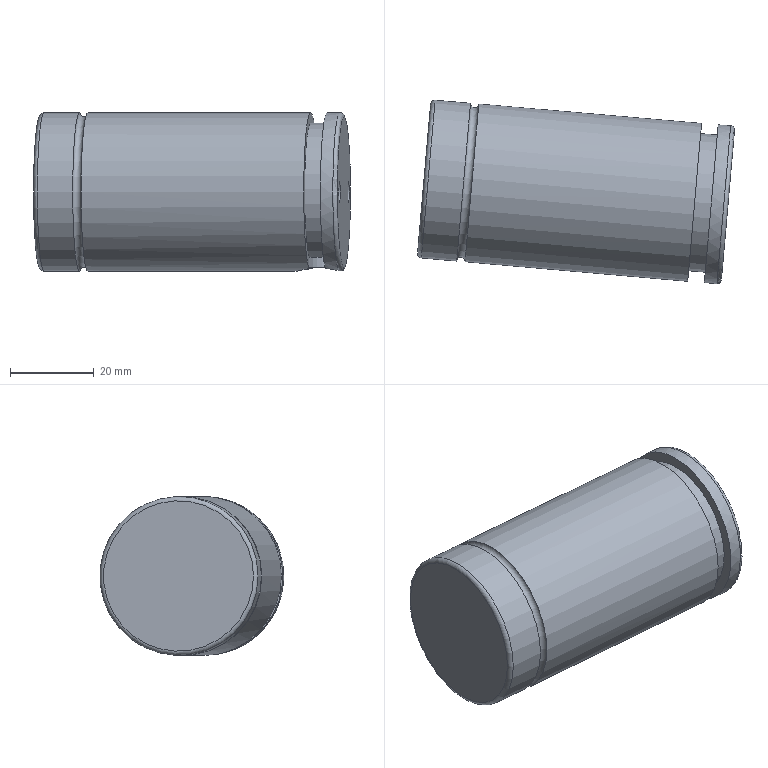Part | NX | features solid 2 | 1 solid | 26 faces | box 75.867 x 44.051 x 38 mm | volume 81103 mm3 | plane 13 | cylinder 8 | torus 3 | cone 2 | commonest cylinder face diameters 38 x3 4.9 x2 9.5 x1 11 x1 33 x1
STEP:
#1=CARTESIAN_POINT('',(-732.743,476.677,-245.));
#2=VERTEX_POINT('',#1);
#3=CARTESIAN_POINT('',(-731.087,495.604,-245.));
#4=DIRECTION('',(-0.9962,0.08716,0.));
#5=DIRECTION('',(-0.08716,-0.9962,0.));
#6=AXIS2_PLACEMENT_3D('',#3,#4,#5);
#7=CIRCLE('',#6,19.);
#8=EDGE_CURVE('',#2,#2,#7,.T.);
#9=ORIENTED_EDGE('',*,*,#8,.T.);
#10=EDGE_LOOP('',(#9));
#11=FACE_BOUND('',#10,.T.);
#12=CARTESIAN_POINT('',(-734.736,476.851,-245.));
#13=VERTEX_POINT('',#12);
#14=CARTESIAN_POINT('',(-733.08,495.779,-245.));
#15=DIRECTION('',(-0.9962,0.08716,0.));
#16=DIRECTION('',(-0.08716,-0.9962,0.));
#17=AXIS2_PLACEMENT_3D('',#14,#15,#16);
#18=CIRCLE('',#17,19.);
#19=EDGE_CURVE('',#13,#13,#18,.T.);
#20=ORIENTED_EDGE('',*,*,#19,.F.);
#21=EDGE_LOOP('',(#20));
#22=FACE_BOUND('',#21,.T.);
#23=CARTESIAN_POINT('',(-732.083,495.692,-245.));
#24=DIRECTION('',(-0.9962,0.08716,0.));
#25=DIRECTION('',(0.,0.,-1.));
#26=AXIS2_PLACEMENT_3D('',#23,#24,#25);
#27=TOROIDAL_SURFACE('',#26,19.,1.);
#28=ADVANCED_FACE('',(#11,#22),#27,.F.);
#29=CARTESIAN_POINT('',(-743.203,477.592,-245.));
#30=VERTEX_POINT('',#29);
#31=CARTESIAN_POINT('',(-741.547,496.52,-245.));
#32=DIRECTION('',(-0.9962,0.08716,0.));
#33=DIRECTION('',(-0.08716,-0.9962,0.));
#34=AXIS2_PLACEMENT_3D('',#31,#32,#33);
#35=CIRCLE('',#34,19.);
#36=EDGE_CURVE('',#30,#30,#35,.T.);
#37=ORIENTED_EDGE('',*,*,#36,.T.);
#38=EDGE_LOOP('',(#37));
#39=FACE_BOUND('',#38,.T.);
#40=CARTESIAN_POINT('',(-744.112,478.675,-245.));
#41=VERTEX_POINT('',#40);
#42=CARTESIAN_POINT('',(-742.543,496.607,-245.));
#43=DIRECTION('',(-0.9962,0.08716,0.));
#44=DIRECTION('',(-0.08716,-0.9962,0.));
#45=AXIS2_PLACEMENT_3D('',#42,#43,#44);
#46=CIRCLE('',#45,18.);
#47=EDGE_CURVE('',#41,#41,#46,.T.);
#48=ORIENTED_EDGE('',*,*,#47,.F.);
#49=EDGE_LOOP('',(#48));
#50=FACE_BOUND('',#49,.T.);
#51=CARTESIAN_POINT('',(-741.547,496.52,-245.));
#52=DIRECTION('',(-0.9962,0.08716,0.));
#53=DIRECTION('',(0.,0.,-1.));
#54=AXIS2_PLACEMENT_3D('',#51,#52,#53);
#55=TOROIDAL_SURFACE('',#54,18.,1.);
#56=ADVANCED_FACE('',(#39,#50),#55,.T.);
#57=ORIENTED_EDGE('',*,*,#19,.T.);
#58=EDGE_LOOP('',(#57));
#59=FACE_BOUND('',#58,.T.);
#60=ORIENTED_EDGE('',*,*,#36,.F.);
#61=EDGE_LOOP('',(#60));
#62=FACE_BOUND('',#61,.T.);
#63=CARTESIAN_POINT('',(-737.313,496.149,-245.));
#64=DIRECTION('',(0.9962,-0.08716,0.));
#65=DIRECTION('',(0.,0.,1.));
#66=AXIS2_PLACEMENT_3D('',#63,#64,#65);
#67=CYLINDRICAL_SURFACE('',#66,19.);
#68=ADVANCED_FACE('',(#59,#62),#67,.T.);
#69=CARTESIAN_POINT('',(-678.237,485.838,-260.684));
#70=VERTEX_POINT('',#69);
#71=CARTESIAN_POINT('',(-677.344,496.046,-260.684));
#72=VERTEX_POINT('',#71);
#73=CARTESIAN_POINT('',(-677.791,490.942,-245.));
#74=DIRECTION('',(-0.9962,0.08716,0.));
#75=DIRECTION('',(-0.08716,-0.9962,0.));
#76=AXIS2_PLACEMENT_3D('',#73,#74,#75);
#77=CIRCLE('',#76,16.5);
#78=EDGE_CURVE('',#70,#72,#77,.T.);
#79=ORIENTED_EDGE('',*,*,#78,.F.);
#80=CARTESIAN_POINT('',(-674.253,485.489,-260.684));
#81=VERTEX_POINT('',#80);
#82=CARTESIAN_POINT('',(-678.237,485.838,-260.684));
#83=CARTESIAN_POINT('',(-677.01,485.23,-260.522));
#84=CARTESIAN_POINT('',(-675.567,485.104,-260.522));
#85=CARTESIAN_POINT('',(-674.253,485.489,-260.684));
#86=B_SPLINE_CURVE_WITH_KNOTS('',3,(#82,#83,#84,#85),.UNSPECIFIED.,.F.,.F.,(4,4),(0.,0.004081),.UNSPECIFIED.);
#87=EDGE_CURVE('',#70,#81,#86,.T.);
#88=ORIENTED_EDGE('',*,*,#87,.T.);
#89=CARTESIAN_POINT('',(-673.36,495.697,-260.684));
#90=VERTEX_POINT('',#89);
#91=CARTESIAN_POINT('',(-673.806,490.593,-245.));
#92=DIRECTION('',(-0.9962,0.08716,0.));
#93=DIRECTION('',(-0.08716,-0.9962,0.));
#94=AXIS2_PLACEMENT_3D('',#91,#92,#93);
#95=CIRCLE('',#94,16.5);
#96=EDGE_CURVE('',#81,#90,#95,.T.);
#97=ORIENTED_EDGE('',*,*,#96,.T.);
#98=CARTESIAN_POINT('',(-673.36,495.697,-260.684));
#99=CARTESIAN_POINT('',(-674.587,496.304,-260.522));
#100=CARTESIAN_POINT('',(-676.03,496.431,-260.522));
#101=CARTESIAN_POINT('',(-677.344,496.046,-260.684));
#102=B_SPLINE_CURVE_WITH_KNOTS('',3,(#98,#99,#100,#101),.UNSPECIFIED.,.F.,.F.,(4,4),(0.,0.004081),.UNSPECIFIED.);
#103=EDGE_CURVE('',#90,#72,#102,.T.);
#104=ORIENTED_EDGE('',*,*,#103,.T.);
#105=EDGE_LOOP('',(#79,#88,#97,#104));
#106=FACE_BOUND('',#105,.T.);
#107=CARTESIAN_POINT('',(-675.798,490.767,-245.));
#108=DIRECTION('',(0.9962,-0.08716,0.));
#109=DIRECTION('',(0.,0.,1.));
#110=AXIS2_PLACEMENT_3D('',#107,#108,#109);
#111=CYLINDRICAL_SURFACE('',#110,16.5);
#112=ADVANCED_FACE('',(#106),#111,.T.);
#113=CARTESIAN_POINT('',(-674.253,485.489,-263.296));
#114=VERTEX_POINT('',#113);
#115=CARTESIAN_POINT('',(-673.36,495.697,-263.296));
#116=VERTEX_POINT('',#115);
#117=CARTESIAN_POINT('',(-673.806,490.593,-245.));
#118=DIRECTION('',(-0.9962,0.08716,0.));
#119=DIRECTION('',(-0.08716,-0.9962,0.));
#120=AXIS2_PLACEMENT_3D('',#117,#118,#119);
#121=CIRCLE('',#120,19.);
#122=EDGE_CURVE('',#114,#116,#121,.T.);
#123=ORIENTED_EDGE('',*,*,#122,.F.);
#124=CARTESIAN_POINT('',(-671.017,488.049,-263.861));
#125=VERTEX_POINT('',#124);
#126=CARTESIAN_POINT('',(-674.253,485.489,-263.296));
#127=CARTESIAN_POINT('',(-672.883,485.89,-263.442));
#128=CARTESIAN_POINT('',(-671.722,486.809,-263.704));
#129=CARTESIAN_POINT('',(-671.017,488.049,-263.861));
#130=B_SPLINE_CURVE_WITH_KNOTS('',3,(#126,#127,#128,#129),.UNSPECIFIED.,.F.,.F.,(4,4),(0.,0.004242),.UNSPECIFIED.);
#131=EDGE_CURVE('',#114,#125,#130,.T.);
#132=ORIENTED_EDGE('',*,*,#131,.T.);
#133=CARTESIAN_POINT('',(-670.618,492.614,-263.861));
#134=VERTEX_POINT('',#133);
#135=CARTESIAN_POINT('',(-670.817,490.331,-245.));
#136=DIRECTION('',(-0.9962,0.08716,0.));
#137=DIRECTION('',(-0.08716,-0.9962,0.));
#138=AXIS2_PLACEMENT_3D('',#135,#136,#137);
#139=CIRCLE('',#138,19.);
#140=EDGE_CURVE('',#125,#134,#139,.T.);
#141=ORIENTED_EDGE('',*,*,#140,.T.);
#142=CARTESIAN_POINT('',(-670.618,492.614,-263.861));
#143=CARTESIAN_POINT('',(-671.097,493.957,-263.704));
#144=CARTESIAN_POINT('',(-672.08,495.064,-263.442));
#145=CARTESIAN_POINT('',(-673.36,495.697,-263.296));
#146=B_SPLINE_CURVE_WITH_KNOTS('',3,(#142,#143,#144,#145),.UNSPECIFIED.,.F.,.F.,(4,4),(0.,0.004242),.UNSPECIFIED.);
#147=EDGE_CURVE('',#134,#116,#146,.T.);
#148=ORIENTED_EDGE('',*,*,#147,.T.);
#149=EDGE_LOOP('',(#123,#132,#141,#148));
#150=FACE_BOUND('',#149,.T.);
#151=CARTESIAN_POINT('',(-672.312,490.462,-245.));
#152=DIRECTION('',(0.9962,-0.08716,0.));
#153=DIRECTION('',(0.,0.,1.));
#154=AXIS2_PLACEMENT_3D('',#151,#152,#153);
#155=CYLINDRICAL_SURFACE('',#154,19.);
#156=ADVANCED_FACE('',(#150),#155,.T.);
#157=CARTESIAN_POINT('',(-670.697,480.233,-245.));
#158=VERTEX_POINT('',#157);
#159=CARTESIAN_POINT('',(-670.911,477.792,-245.));
#160=DIRECTION('',(-0.9962,0.08716,0.));
#161=DIRECTION('',(0.08716,0.9962,0.));
#162=AXIS2_PLACEMENT_3D('',#159,#160,#161);
#163=CIRCLE('',#162,2.45);
#164=EDGE_CURVE('',#158,#158,#163,.T.);
#165=ORIENTED_EDGE('',*,*,#164,.F.);
#166=EDGE_LOOP('',(#165));
#167=FACE_BOUND('',#166,.T.);
#168=CARTESIAN_POINT('',(-677.87,480.86,-245.));
#169=VERTEX_POINT('',#168);
#170=CARTESIAN_POINT('',(-678.083,478.419,-245.));
#171=DIRECTION('',(0.9962,-0.08716,0.));
#172=DIRECTION('',(0.08716,0.9962,0.));
#173=AXIS2_PLACEMENT_3D('',#170,#171,#172);
#174=CIRCLE('',#173,2.45);
#175=EDGE_CURVE('',#169,#169,#174,.T.);
#176=ORIENTED_EDGE('',*,*,#175,.F.);
#177=EDGE_LOOP('',(#176));
#178=FACE_BOUND('',#177,.T.);
#179=CARTESIAN_POINT('',(-674.497,478.106,-245.));
#180=DIRECTION('',(-0.9962,0.08716,0.));
#181=DIRECTION('',(0.,0.,-1.));
#182=AXIS2_PLACEMENT_3D('',#179,#180,#181);
#183=CYLINDRICAL_SURFACE('',#182,2.45);
#184=ADVANCED_FACE('',(#167,#178),#183,.F.);
#185=CARTESIAN_POINT('',(-679.378,478.533,-245.));
#186=VERTEX_POINT('',#185);
#187=VERTEX_LOOP('',#186);
#188=FACE_BOUND('',#187,.T.);
#189=ORIENTED_EDGE('',*,*,#175,.T.);
#190=EDGE_LOOP('',(#189));
#191=FACE_BOUND('',#190,.T.);
#192=CARTESIAN_POINT('',(-678.731,478.476,-245.));
#193=DIRECTION('',(0.9962,-0.08716,0.));
#194=DIRECTION('',(0.,0.,1.));
#195=AXIS2_PLACEMENT_3D('',#192,#193,#194);
#196=CONICAL_SURFACE('',#195,1.225,1.083);
#197=ADVANCED_FACE('',(#188,#191),#196,.F.);
#198=CARTESIAN_POINT('',(-676.118,500.884,-245.));
#199=VERTEX_POINT('',#198);
#200=CARTESIAN_POINT('',(-675.904,503.324,-245.));
#201=DIRECTION('',(-0.9962,0.08716,0.));
#202=DIRECTION('',(-0.08716,-0.9962,0.));
#203=AXIS2_PLACEMENT_3D('',#200,#201,#202);
#204=CIRCLE('',#203,2.45);
#205=EDGE_CURVE('',#199,#199,#204,.T.);
#206=ORIENTED_EDGE('',*,*,#205,.F.);
#207=EDGE_LOOP('',(#206));
#208=FACE_BOUND('',#207,.T.);
#209=CARTESIAN_POINT('',(-677.199,503.438,-245.));
#210=VERTEX_POINT('',#209);
#211=VERTEX_LOOP('',#210);
#212=FACE_BOUND('',#211,.T.);
#213=CARTESIAN_POINT('',(-676.552,503.381,-245.));
#214=DIRECTION('',(0.9962,-0.08716,0.));
#215=DIRECTION('',(0.,0.,1.));
#216=AXIS2_PLACEMENT_3D('',#213,#214,#215);
#217=CONICAL_SURFACE('',#216,1.225,1.083);
#218=ADVANCED_FACE('',(#208,#212),#217,.F.);
#219=ORIENTED_EDGE('',*,*,#205,.T.);
#220=EDGE_LOOP('',(#219));
#221=FACE_BOUND('',#220,.T.);
#222=CARTESIAN_POINT('',(-668.945,500.256,-245.));
#223=VERTEX_POINT('',#222);
#224=CARTESIAN_POINT('',(-668.732,502.697,-245.));
#225=DIRECTION('',(-0.9962,0.08716,0.));
#226=DIRECTION('',(-0.08716,-0.9962,0.));
#227=AXIS2_PLACEMENT_3D('',#224,#225,#226);
#228=CIRCLE('',#227,2.45);
#229=EDGE_CURVE('',#223,#223,#228,.T.);
#230=ORIENTED_EDGE('',*,*,#229,.F.);
#231=EDGE_LOOP('',(#230));
#232=FACE_BOUND('',#231,.T.);
#233=CARTESIAN_POINT('',(-672.318,503.01,-245.));
#234=DIRECTION('',(0.9962,-0.08716,0.));
#235=DIRECTION('',(0.,0.,1.));
#236=AXIS2_PLACEMENT_3D('',#233,#234,#235);
#237=CYLINDRICAL_SURFACE('',#236,2.45);
#238=ADVANCED_FACE('',(#221,#232),#237,.F.);
#239=CARTESIAN_POINT('',(-671.39,472.313,-245.));
#240=VERTEX_POINT('',#239);
#241=CARTESIAN_POINT('',(-669.821,490.244,-245.));
#242=DIRECTION('',(-0.9962,0.08716,0.));
#243=DIRECTION('',(-0.08716,-0.9962,0.));
#244=AXIS2_PLACEMENT_3D('',#241,#242,#243);
#245=CIRCLE('',#244,18.);
#246=EDGE_CURVE('',#240,#240,#245,.T.);
#247=ORIENTED_EDGE('',*,*,#246,.T.);
#248=EDGE_LOOP('',(#247));
#249=FACE_BOUND('',#248,.T.);
#250=CARTESIAN_POINT('',(-671.017,488.049,-263.861));
#251=CARTESIAN_POINT('',(-670.626,488.737,-263.949));
#252=CARTESIAN_POINT('',(-670.15,490.274,-263.783));
#253=CARTESIAN_POINT('',(-670.352,491.868,-263.949));
#254=CARTESIAN_POINT('',(-670.618,492.614,-263.861));
#255=B_SPLINE_CURVE_WITH_KNOTS('',3,(#250,#251,#252,#253,#254),.UNSPECIFIED.,.F.,.F.,(4,1,4),(0.,0.002357,0.004713),.UNSPECIFIED.);
#256=EDGE_CURVE('',#125,#134,#255,.T.);
#257=ORIENTED_EDGE('',*,*,#256,.T.);
#258=ORIENTED_EDGE('',*,*,#140,.F.);
#259=EDGE_LOOP('',(#257,#258));
#260=FACE_BOUND('',#259,.T.);
#261=CARTESIAN_POINT('',(-670.817,490.331,-245.));
#262=DIRECTION('',(-0.9962,0.08716,0.));
#263=DIRECTION('',(0.,0.,-1.));
#264=AXIS2_PLACEMENT_3D('',#261,#262,#263);
#265=TOROIDAL_SURFACE('',#264,18.,1.);
#266=ADVANCED_FACE('',(#249,#260),#265,.T.);
#267=CARTESIAN_POINT('',(-678.237,485.838,-263.296));
#268=VERTEX_POINT('',#267);
#269=CARTESIAN_POINT('',(-677.344,496.046,-263.296));
#270=VERTEX_POINT('',#269);
#271=CARTESIAN_POINT('',(-677.791,490.942,-245.));
#272=DIRECTION('',(-0.9962,0.08716,0.));
#273=DIRECTION('',(-0.08716,-0.9962,0.));
#274=AXIS2_PLACEMENT_3D('',#271,#272,#273);
#275=CIRCLE('',#274,19.);
#276=EDGE_CURVE('',#268,#270,#275,.T.);
#277=ORIENTED_EDGE('',*,*,#276,.T.);
#278=CARTESIAN_POINT('',(-677.344,496.046,-263.296));
#279=CARTESIAN_POINT('',(-678.409,495.734,-263.409));
#280=CARTESIAN_POINT('',(-680.292,494.49,-263.782));
#281=CARTESIAN_POINT('',(-681.623,491.275,-264.109));
#282=CARTESIAN_POINT('',(-680.879,487.899,-263.784));
#283=CARTESIAN_POINT('',(-679.232,486.33,-263.409));
#284=CARTESIAN_POINT('',(-678.237,485.838,-263.296));
#285=B_SPLINE_CURVE_WITH_KNOTS('',3,(#278,#279,#280,#281,#282,#283,#284),.UNSPECIFIED.,.F.,.F.,(4,1,1,1,4),(-0.006599,-0.0033,-0.000001213,0.003297,0.006596),.UNSPECIFIED.);
#286=EDGE_CURVE('',#270,#268,#285,.T.);
#287=ORIENTED_EDGE('',*,*,#286,.T.);
#288=EDGE_LOOP('',(#277,#287));
#289=FACE_BOUND('',#288,.T.);
#290=ORIENTED_EDGE('',*,*,#8,.F.);
#291=EDGE_LOOP('',(#290));
#292=FACE_BOUND('',#291,.T.);
#293=CARTESIAN_POINT('',(-704.439,493.273,-245.));
#294=DIRECTION('',(0.9962,-0.08716,0.));
#295=DIRECTION('',(0.,0.,1.));
#296=AXIS2_PLACEMENT_3D('',#293,#294,#295);
#297=CYLINDRICAL_SURFACE('',#296,19.);
#298=ADVANCED_FACE('',(#289,#292),#297,.T.);
#299=CARTESIAN_POINT('',(-676.278,485.288,-260.5));
#300=VERTEX_POINT('',#299);
#301=CARTESIAN_POINT('',(-675.798,490.767,-260.5));
#302=DIRECTION('',(0.,0.,-1.));
#303=DIRECTION('',(-0.08716,-0.9962,0.));
#304=AXIS2_PLACEMENT_3D('',#301,#302,#303);
#305=CIRCLE('',#304,5.5);
#306=EDGE_CURVE('',#300,#300,#305,.T.);
#307=ORIENTED_EDGE('',*,*,#306,.F.);
#308=EDGE_LOOP('',(#307));
#309=FACE_BOUND('',#308,.T.);
#310=ORIENTED_EDGE('',*,*,#87,.F.);
#311=CARTESIAN_POINT('',(-678.237,485.838,-262.25));
#312=DIRECTION('',(0.,0.,1.));
#313=VECTOR('',#312,1000.);
#314=LINE('',#311,#313);
#315=EDGE_CURVE('',#268,#70,#314,.T.);
#316=ORIENTED_EDGE('',*,*,#315,.F.);
#317=ORIENTED_EDGE('',*,*,#286,.F.);
#318=CARTESIAN_POINT('',(-677.344,496.046,-262.25));
#319=DIRECTION('',(0.,0.,-1.));
#320=VECTOR('',#319,1000.);
#321=LINE('',#318,#320);
#322=EDGE_CURVE('',#72,#270,#321,.T.);
#323=ORIENTED_EDGE('',*,*,#322,.F.);
#324=ORIENTED_EDGE('',*,*,#103,.F.);
#325=CARTESIAN_POINT('',(-673.36,495.697,-262.25));
#326=DIRECTION('',(0.,0.,1.));
#327=VECTOR('',#326,1000.);
#328=LINE('',#325,#327);
#329=EDGE_CURVE('',#116,#90,#328,.T.);
#330=ORIENTED_EDGE('',*,*,#329,.F.);
#331=ORIENTED_EDGE('',*,*,#147,.F.);
#332=ORIENTED_EDGE('',*,*,#256,.F.);
#333=ORIENTED_EDGE('',*,*,#131,.F.);
#334=CARTESIAN_POINT('',(-674.253,485.489,-262.25));
#335=DIRECTION('',(0.,0.,-1.));
#336=VECTOR('',#335,1000.);
#337=LINE('',#334,#336);
#338=EDGE_CURVE('',#81,#114,#337,.T.);
#339=ORIENTED_EDGE('',*,*,#338,.F.);
#340=EDGE_LOOP('',(#310,#316,#317,#323,#324,#330,#331,#332,#333,#339));
#341=FACE_BOUND('',#340,.T.);
#342=CARTESIAN_POINT('',(-675.798,490.767,-264.));
#343=DIRECTION('',(0.,0.,-1.));
#344=DIRECTION('',(-0.08716,-0.9962,0.));
#345=AXIS2_PLACEMENT_3D('',#342,#343,#344);
#346=CYLINDRICAL_SURFACE('',#345,5.5);
#347=ADVANCED_FACE('',(#309,#341),#346,.F.);
#348=CARTESIAN_POINT('',(-676.212,486.035,-260.5));
#349=VERTEX_POINT('',#348);
#350=CARTESIAN_POINT('',(-675.798,490.767,-260.5));
#351=DIRECTION('',(0.,0.,1.));
#352=DIRECTION('',(-0.08716,-0.9962,0.));
#353=AXIS2_PLACEMENT_3D('',#350,#351,#352);
#354=CIRCLE('',#353,4.75);
#355=EDGE_CURVE('',#349,#349,#354,.T.);
#356=ORIENTED_EDGE('',*,*,#355,.F.);
#357=EDGE_LOOP('',(#356));
#358=FACE_BOUND('',#357,.T.);
#359=CARTESIAN_POINT('',(-676.212,486.035,-263.));
#360=VERTEX_POINT('',#359);
#361=CARTESIAN_POINT('',(-675.798,490.767,-263.));
#362=DIRECTION('',(0.,0.,1.));
#363=DIRECTION('',(-0.08716,-0.9962,0.));
#364=AXIS2_PLACEMENT_3D('',#361,#362,#363);
#365=CIRCLE('',#364,4.75);
#366=EDGE_CURVE('',#360,#360,#365,.T.);
#367=ORIENTED_EDGE('',*,*,#366,.T.);
#368=EDGE_LOOP('',(#367));
#369=FACE_BOUND('',#368,.T.);
#370=CARTESIAN_POINT('',(-675.798,490.767,-245.));
#371=DIRECTION('',(0.,0.,1.));
#372=DIRECTION('',(0.08716,0.9962,0.));
#373=AXIS2_PLACEMENT_3D('',#370,#371,#372);
#374=CYLINDRICAL_SURFACE('',#373,4.75);
#375=ADVANCED_FACE('',(#358,#369),#374,.T.);
#376=CARTESIAN_POINT('',(-674.805,492.186,-260.));
#377=VERTEX_POINT('',#376);
#378=CARTESIAN_POINT('',(-674.073,490.616,-260.));
#379=VERTEX_POINT('',#378);
#380=CARTESIAN_POINT('',(-674.805,492.186,-260.));
#381=DIRECTION('',(0.4226,-0.9063,0.));
#382=VECTOR('',#381,1000.);
#383=LINE('',#380,#382);
#384=EDGE_CURVE('',#377,#379,#383,.T.);
#385=ORIENTED_EDGE('',*,*,#384,.F.);
#386=CARTESIAN_POINT('',(-674.805,492.186,-263.));
#387=VERTEX_POINT('',#386);
#388=CARTESIAN_POINT('',(-674.805,492.186,-263.));
#389=DIRECTION('',(0.,0.,1.));
#390=VECTOR('',#389,1000.);
#391=LINE('',#388,#390);
#392=EDGE_CURVE('',#387,#377,#391,.T.);
#393=ORIENTED_EDGE('',*,*,#392,.F.);
#394=CARTESIAN_POINT('',(-674.073,490.616,-263.));
#395=VERTEX_POINT('',#394);
#396=CARTESIAN_POINT('',(-673.988,490.434,-263.));
#397=DIRECTION('',(-0.4226,0.9063,0.));
#398=VECTOR('',#397,1000.);
#399=LINE('',#396,#398);
#400=EDGE_CURVE('',#395,#387,#399,.T.);
#401=ORIENTED_EDGE('',*,*,#400,.F.);
#402=CARTESIAN_POINT('',(-674.073,490.616,-263.));
#403=DIRECTION('',(0.,0.,1.));
#404=VECTOR('',#403,1000.);
#405=LINE('',#402,#404);
#406=EDGE_CURVE('',#395,#379,#405,.T.);
#407=ORIENTED_EDGE('',*,*,#406,.T.);
#408=EDGE_LOOP('',(#385,#393,#401,#407));
#409=FACE_BOUND('',#408,.T.);
#410=CARTESIAN_POINT('',(-674.805,492.186,-263.));
#411=DIRECTION('',(0.9063,0.4226,0.));
#412=DIRECTION('',(0.4226,-0.9063,0.));
#413=AXIS2_PLACEMENT_3D('',#410,#411,#412);
#414=PLANE('',#413);
#415=ADVANCED_FACE('',(#409),#414,.F.);
#416=CARTESIAN_POINT('',(-675.066,489.197,-260.));
#417=VERTEX_POINT('',#416);
#418=CARTESIAN_POINT('',(-674.073,490.616,-260.));
#419=DIRECTION('',(-0.5736,-0.8192,0.));
#420=VECTOR('',#419,1000.);
#421=LINE('',#418,#420);
#422=EDGE_CURVE('',#379,#417,#421,.T.);
#423=ORIENTED_EDGE('',*,*,#422,.F.);
#424=ORIENTED_EDGE('',*,*,#406,.F.);
#425=CARTESIAN_POINT('',(-675.066,489.197,-263.));
#426=VERTEX_POINT('',#425);
#427=CARTESIAN_POINT('',(-673.461,491.49,-263.));
#428=DIRECTION('',(0.5736,0.8192,0.));
#429=VECTOR('',#428,1000.);
#430=LINE('',#427,#429);
#431=EDGE_CURVE('',#426,#395,#430,.T.);
#432=ORIENTED_EDGE('',*,*,#431,.F.);
#433=CARTESIAN_POINT('',(-675.066,489.197,-263.));
#434=DIRECTION('',(0.,0.,1.));
#435=VECTOR('',#434,1000.);
#436=LINE('',#433,#435);
#437=EDGE_CURVE('',#426,#417,#436,.T.);
#438=ORIENTED_EDGE('',*,*,#437,.T.);
#439=EDGE_LOOP('',(#423,#424,#432,#438));
#440=FACE_BOUND('',#439,.T.);
#441=CARTESIAN_POINT('',(-674.073,490.616,-263.));
#442=DIRECTION('',(0.8192,-0.5736,0.));
#443=DIRECTION('',(-0.5736,-0.8192,0.));
#444=AXIS2_PLACEMENT_3D('',#441,#442,#443);
#445=PLANE('',#444);
#446=ADVANCED_FACE('',(#440),#445,.F.);
#447=CARTESIAN_POINT('',(-676.792,489.348,-260.));
#448=VERTEX_POINT('',#447);
#449=CARTESIAN_POINT('',(-675.066,489.197,-260.));
#450=DIRECTION('',(-0.9962,0.08716,0.));
#451=VECTOR('',#450,1000.);
#452=LINE('',#449,#451);
#453=EDGE_CURVE('',#417,#448,#452,.T.);
#454=ORIENTED_EDGE('',*,*,#453,.F.);
#455=ORIENTED_EDGE('',*,*,#437,.F.);
#456=CARTESIAN_POINT('',(-676.792,489.348,-263.));
#457=VERTEX_POINT('',#456);
#458=CARTESIAN_POINT('',(-672.509,488.974,-263.));
#459=DIRECTION('',(0.9962,-0.08716,0.));
#460=VECTOR('',#459,1000.);
#461=LINE('',#458,#460);
#462=EDGE_CURVE('',#457,#426,#461,.T.);
#463=ORIENTED_EDGE('',*,*,#462,.F.);
#464=CARTESIAN_POINT('',(-676.792,489.348,-263.));
#465=DIRECTION('',(0.,0.,1.));
#466=VECTOR('',#465,1000.);
#467=LINE('',#464,#466);
#468=EDGE_CURVE('',#457,#448,#467,.T.);
#469=ORIENTED_EDGE('',*,*,#468,.T.);
#470=EDGE_LOOP('',(#454,#455,#463,#469));
#471=FACE_BOUND('',#470,.T.);
#472=CARTESIAN_POINT('',(-675.066,489.197,-263.));
#473=DIRECTION('',(-0.08716,-0.9962,0.));
#474=DIRECTION('',(0.,0.,1.));
#475=AXIS2_PLACEMENT_3D('',#472,#473,#474);
#476=PLANE('',#475);
#477=ADVANCED_FACE('',(#471),#476,.F.);
#478=CARTESIAN_POINT('',(-677.524,490.918,-260.));
#479=VERTEX_POINT('',#478);
#480=CARTESIAN_POINT('',(-676.792,489.348,-260.));
#481=DIRECTION('',(-0.4226,0.9063,0.));
#482=VECTOR('',#481,1000.);
#483=LINE('',#480,#482);
#484=EDGE_CURVE('',#448,#479,#483,.T.);
#485=ORIENTED_EDGE('',*,*,#484,.F.);
#486=ORIENTED_EDGE('',*,*,#468,.F.);
#487=CARTESIAN_POINT('',(-677.524,490.918,-263.));
#488=VERTEX_POINT('',#487);
#489=CARTESIAN_POINT('',(-676.341,488.381,-263.));
#490=DIRECTION('',(0.4226,-0.9063,0.));
#491=VECTOR('',#490,1000.);
#492=LINE('',#489,#491);
#493=EDGE_CURVE('',#488,#457,#492,.T.);
#494=ORIENTED_EDGE('',*,*,#493,.F.);
#495=CARTESIAN_POINT('',(-677.524,490.918,-263.));
#496=DIRECTION('',(0.,0.,1.));
#497=VECTOR('',#496,1000.);
#498=LINE('',#495,#497);
#499=EDGE_CURVE('',#488,#479,#498,.T.);
#500=ORIENTED_EDGE('',*,*,#499,.T.);
#501=EDGE_LOOP('',(#485,#486,#494,#500));
#502=FACE_BOUND('',#501,.T.);
#503=CARTESIAN_POINT('',(-676.792,489.348,-263.));
#504=DIRECTION('',(-0.9063,-0.4226,0.));
#505=DIRECTION('',(-0.4226,0.9063,0.));
#506=AXIS2_PLACEMENT_3D('',#503,#504,#505);
#507=PLANE('',#506);
#508=ADVANCED_FACE('',(#502),#507,.F.);
#509=CARTESIAN_POINT('',(-676.53,492.337,-260.));
#510=VERTEX_POINT('',#509);
#511=CARTESIAN_POINT('',(-677.524,490.918,-260.));
#512=DIRECTION('',(0.5736,0.8192,0.));
#513=VECTOR('',#512,1000.);
#514=LINE('',#511,#513);
#515=EDGE_CURVE('',#479,#510,#514,.T.);
#516=ORIENTED_EDGE('',*,*,#515,.F.);
#517=ORIENTED_EDGE('',*,*,#499,.F.);
#518=CARTESIAN_POINT('',(-676.53,492.337,-263.));
#519=VERTEX_POINT('',#518);
#520=CARTESIAN_POINT('',(-676.415,492.502,-263.));
#521=DIRECTION('',(-0.5736,-0.8192,0.));
#522=VECTOR('',#521,1000.);
#523=LINE('',#520,#522);
#524=EDGE_CURVE('',#519,#488,#523,.T.);
#525=ORIENTED_EDGE('',*,*,#524,.F.);
#526=CARTESIAN_POINT('',(-676.53,492.337,-263.));
#527=DIRECTION('',(0.,0.,1.));
#528=VECTOR('',#527,1000.);
#529=LINE('',#526,#528);
#530=EDGE_CURVE('',#519,#510,#529,.T.);
#531=ORIENTED_EDGE('',*,*,#530,.T.);
#532=EDGE_LOOP('',(#516,#517,#525,#531));
#533=FACE_BOUND('',#532,.T.);
#534=CARTESIAN_POINT('',(-677.524,490.918,-263.));
#535=DIRECTION('',(-0.8192,0.5736,0.));
#536=DIRECTION('',(0.5736,0.8192,0.));
#537=AXIS2_PLACEMENT_3D('',#534,#535,#536);
#538=PLANE('',#537);
#539=ADVANCED_FACE('',(#533),#538,.F.);
#540=CARTESIAN_POINT('',(-676.53,492.337,-260.));
#541=DIRECTION('',(0.9962,-0.08716,0.));
#542=VECTOR('',#541,1000.);
#543=LINE('',#540,#542);
#544=EDGE_CURVE('',#510,#377,#543,.T.);
#545=ORIENTED_EDGE('',*,*,#544,.F.);
#546=ORIENTED_EDGE('',*,*,#530,.F.);
#547=CARTESIAN_POINT('',(-673.11,492.038,-263.));
#548=DIRECTION('',(-0.9962,0.08716,0.));
#549=VECTOR('',#548,1000.);
#550=LINE('',#547,#549);
#551=EDGE_CURVE('',#387,#519,#550,.T.);
#552=ORIENTED_EDGE('',*,*,#551,.F.);
#553=ORIENTED_EDGE('',*,*,#392,.T.);
#554=EDGE_LOOP('',(#545,#546,#552,#553));
#555=FACE_BOUND('',#554,.T.);
#556=CARTESIAN_POINT('',(-676.53,492.337,-263.));
#557=DIRECTION('',(0.08716,0.9962,0.));
#558=DIRECTION('',(0.,0.,-1.));
#559=AXIS2_PLACEMENT_3D('',#556,#557,#558);
#560=PLANE('',#559);
#561=ADVANCED_FACE('',(#555),#560,.F.);
#562=ORIENTED_EDGE('',*,*,#384,.T.);
#563=ORIENTED_EDGE('',*,*,#422,.T.);
#564=ORIENTED_EDGE('',*,*,#453,.T.);
#565=ORIENTED_EDGE('',*,*,#484,.T.);
#566=ORIENTED_EDGE('',*,*,#515,.T.);
#567=ORIENTED_EDGE('',*,*,#544,.T.);
#568=EDGE_LOOP('',(#562,#563,#564,#565,#566,#567));
#569=FACE_BOUND('',#568,.T.);
#570=CARTESIAN_POINT('',(-675.798,490.767,-260.));
#571=DIRECTION('',(0.,0.,-1.));
#572=DIRECTION('',(-0.08716,-0.9962,0.));
#573=AXIS2_PLACEMENT_3D('',#570,#571,#572);
#574=PLANE('',#573);
#575=ADVANCED_FACE('',(#569),#574,.T.);
#576=ORIENTED_EDGE('',*,*,#400,.T.);
#577=ORIENTED_EDGE('',*,*,#551,.T.);
#578=ORIENTED_EDGE('',*,*,#524,.T.);
#579=ORIENTED_EDGE('',*,*,#493,.T.);
#580=ORIENTED_EDGE('',*,*,#462,.T.);
#581=ORIENTED_EDGE('',*,*,#431,.T.);
#582=EDGE_LOOP('',(#576,#577,#578,#579,#580,#581));
#583=FACE_BOUND('',#582,.T.);
#584=ORIENTED_EDGE('',*,*,#366,.F.);
#585=EDGE_LOOP('',(#584));
#586=FACE_BOUND('',#585,.T.);
#587=CARTESIAN_POINT('',(-669.821,490.244,-263.));
#588=DIRECTION('',(0.,0.,-1.));
#589=DIRECTION('',(-0.08716,-0.9962,0.));
#590=AXIS2_PLACEMENT_3D('',#587,#588,#589);
#591=PLANE('',#590);
#592=ADVANCED_FACE('',(#583,#586),#591,.T.);
#593=ORIENTED_EDGE('',*,*,#355,.T.);
#594=EDGE_LOOP('',(#593));
#595=FACE_BOUND('',#594,.T.);
#596=ORIENTED_EDGE('',*,*,#306,.T.);
#597=EDGE_LOOP('',(#596));
#598=FACE_BOUND('',#597,.T.);
#599=CARTESIAN_POINT('',(-669.821,490.244,-260.5));
#600=DIRECTION('',(0.,0.,-1.));
#601=DIRECTION('',(-0.08716,-0.9962,0.));
#602=AXIS2_PLACEMENT_3D('',#599,#600,#601);
#603=PLANE('',#602);
#604=ADVANCED_FACE('',(#595,#598),#603,.T.);
#605=ORIENTED_EDGE('',*,*,#229,.T.);
#606=EDGE_LOOP('',(#605));
#607=FACE_BOUND('',#606,.T.);
#608=ORIENTED_EDGE('',*,*,#164,.T.);
#609=EDGE_LOOP('',(#608));
#610=FACE_BOUND('',#609,.T.);
#611=ORIENTED_EDGE('',*,*,#246,.F.);
#612=EDGE_LOOP('',(#611));
#613=FACE_BOUND('',#612,.T.);
#614=CARTESIAN_POINT('',(-670.606,481.279,-245.));
#615=DIRECTION('',(0.9962,-0.08716,0.));
#616=DIRECTION('',(-0.08716,-0.9962,0.));
#617=AXIS2_PLACEMENT_3D('',#614,#615,#616);
#618=PLANE('',#617);
#619=ADVANCED_FACE('',(#607,#610,#613),#618,.T.);
#620=ORIENTED_EDGE('',*,*,#329,.T.);
#621=ORIENTED_EDGE('',*,*,#96,.F.);
#622=ORIENTED_EDGE('',*,*,#338,.T.);
#623=ORIENTED_EDGE('',*,*,#122,.T.);
#624=EDGE_LOOP('',(#620,#621,#622,#623));
#625=FACE_BOUND('',#624,.T.);
#626=CARTESIAN_POINT('',(-675.353,472.91,-245.));
#627=DIRECTION('',(-0.9962,0.08716,0.));
#628=DIRECTION('',(0.,0.,-1.));
#629=AXIS2_PLACEMENT_3D('',#626,#627,#628);
#630=PLANE('',#629);
#631=ADVANCED_FACE('',(#625),#630,.T.);
#632=ORIENTED_EDGE('',*,*,#322,.T.);
#633=ORIENTED_EDGE('',*,*,#276,.F.);
#634=ORIENTED_EDGE('',*,*,#315,.T.);
#635=ORIENTED_EDGE('',*,*,#78,.T.);
#636=EDGE_LOOP('',(#632,#633,#634,#635));
#637=FACE_BOUND('',#636,.T.);
#638=CARTESIAN_POINT('',(-679.338,473.259,-245.));
#639=DIRECTION('',(0.9962,-0.08716,0.));
#640=DIRECTION('',(0.,0.,1.));
#641=AXIS2_PLACEMENT_3D('',#638,#639,#640);
#642=PLANE('',#641);
#643=ADVANCED_FACE('',(#637),#642,.T.);
#644=ORIENTED_EDGE('',*,*,#47,.T.);
#645=EDGE_LOOP('',(#644));
#646=FACE_BOUND('',#645,.T.);
#647=CARTESIAN_POINT('',(-743.328,487.641,-245.));
#648=DIRECTION('',(-0.9962,0.08716,0.));
#649=DIRECTION('',(0.,0.,-1.));
#650=AXIS2_PLACEMENT_3D('',#647,#648,#649);
#651=PLANE('',#650);
#652=ADVANCED_FACE('',(#646),#651,.T.);
#653=CLOSED_SHELL('',(#28,#56,#68,#112,#156,#184,#197,#218,#238,#266,#298,#347,#375,#415,#446,#477,#508,#539,#561,#575,#592,#604,#619,#631,#643,#652));
#654=MANIFOLD_SOLID_BREP('',#653);
#655=(LENGTH_UNIT()NAMED_UNIT(*)SI_UNIT(.MILLI.,.METRE.));
#656=UNCERTAINTY_MEASURE_WITH_UNIT(LENGTH_MEASURE(0.0508),#655,'','');
#657=(NAMED_UNIT(*)PLANE_ANGLE_UNIT()SI_UNIT($,.RADIAN.));
#658=(NAMED_UNIT(*)SI_UNIT($,.STERADIAN.)SOLID_ANGLE_UNIT());
#659=(GEOMETRIC_REPRESENTATION_CONTEXT(3)GLOBAL_UNCERTAINTY_ASSIGNED_CONTEXT((#656))GLOBAL_UNIT_ASSIGNED_CONTEXT((#655,#657,#658))REPRESENTATION_CONTEXT('',''));
#660=ADVANCED_BREP_SHAPE_REPRESENTATION('',(#654),#659);